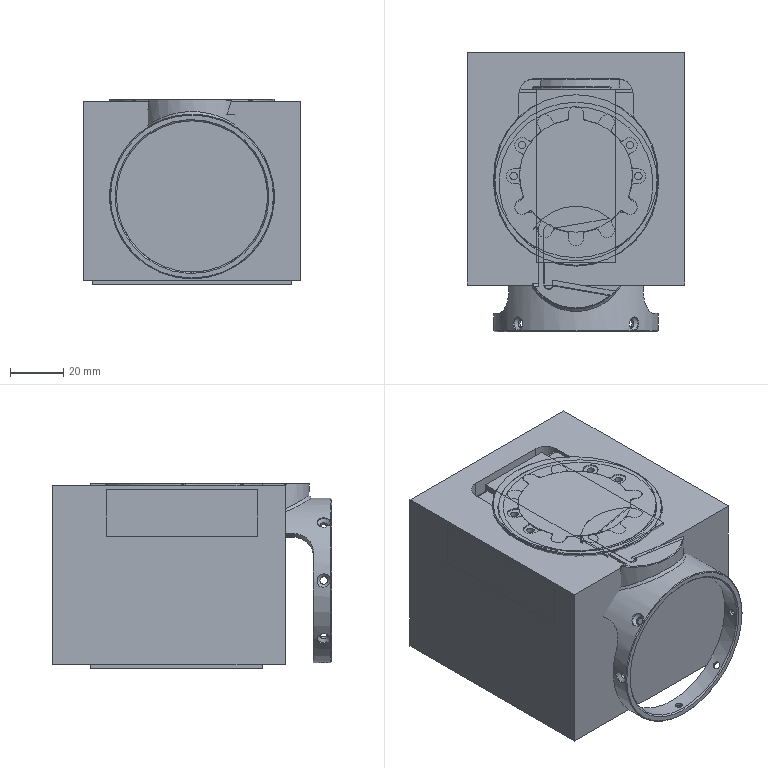NC program | NX | posted with a generic post | part box 82 x 105.2 x 70 mm
Lines 1 to 900 of 123648:
N10 G17 G21 G94 G90
(单向轮廓精光_2 , TOOL : 飞刀D50)
N12 T20 M6
N14 G53
N16 G17 G0 G90 X-63.629 Y-5.85 S5500 M3
N18 G43 Z40.05 H20
N20 Z3.05
N22 G94 G1 Z0.05 F800.
N24 G41 X-51.5 D20
N26 G3 X-48.5 Y-2.85 R3.
N28 G2 X0. Y45.65 R48.5
N30 X-48.5 Y-2.85 R-48.5
N32 X-48.497 Y-2.35 R48.5
N34 G3 X-51.466 Y0.681 R3.
N36 G1 X-63.395 Y0.804
N38 G40
N40 X-63.595 Y0.806
N42 Z3.05
N44 G0 Z40.05
N46 M5
(外形动态铣 , TOOL : 粗刀D16)
N48 T18 M6
N50 G53
N52 G17 G0 G90 X-43.842 Y-2.841 S8500 M3
N54 G43 Z43.08 H18
N56 G94 G1 Z-36.92 F4500.
N58 Z-37.92
N60 X-41.377 Y-3.256
N62 G3 X-40.531 Y-2.841 R0.808
N64 X-40.076 Y-1.778 R5.051
N66 X-39.508 Y1.018 R16.6
N68 X-39.175 Y5.411 R51.899
N70 X-39.062 Y10.142 R137.49
N72 X-39. Y23.191 R842.38
N74 G1 X-38.997 Y33.828
N76 G2 X-38.706 Y36.242 R9.777
N78 X-36.994 Y39.327 R7.332
N80 X-34.009 Y41.563 R10.476
N82 X-30.312 Y42.892 R16.459
N84 X-25.684 Y43.606 R32.132
N86 X-19.505 Y43.912 R90.843
N88 X-7.131 Y43.999 R599.853
N90 G1 X28.819 Y43.997
N92 G2 X31.234 Y43.711 R10.059
N94 X34.021 Y42.218 R7.173
N96 X36.263 Y39.468 R10.133
N98 X37.731 Y35.826 R15.468
N100 X38.524 Y31.402 R28.5
N102 X38.891 Y25.227 R77.968
N104 X38.996 Y14.54 R445.482
N106 G1 X38.999 Y0.986
N108 G2 X39.12 Y-5.181 R38.622
N110 G3 X39.011 Y-14.829 R391.76
N112 G2 X39.006 Y-18.198 R174.731
N114 G1 X38.996 Y-33.89
N116 G2 X38.692 Y-36.301 R9.598
N118 X37.289 Y-38.928 R7.164
N120 X34.571 Y-41.203 R10.136
N122 X31.121 Y-42.648 R15.035
N124 X26.703 Y-43.49 R27.258
N126 X21.28 Y-43.858 R66.36
N128 X13.594 Y-43.983 R258.777
N130 X5.719 Y-43.999 R1000.
N132 G1 X-28.731 Y-43.998
N134 G2 X-31.149 Y-43.735 R10.493
N136 X-34.096 Y-42.155 R7.16
N138 X-36.217 Y-39.55 R10.128
N140 X-37.709 Y-35.911 R15.308
N142 X-38.515 Y-31.489 R28.138
N144 X-38.878 Y-25.689 R73.44
N146 X-38.985 Y-18.378 R277.454
N148 X-38.992 Y-7.74 R1000.
N150 G1 X-38.962 Y-7.053
N152 G2 X-38.286 Y5.503 R39.004
N154 G3 X-37.805 Y9.676 R36.79
N156 X-37.638 Y13.604 R77.844
N158 X-37.516 Y21.71 R298.384
N160 X-37.498 Y30.316 R1000.
N162 G2 X-37.024 Y33.454 R9.775
N164 X-34.408 Y37.509 R9.889
N166 X-30.998 Y39.83 R13.575
N168 X-26.565 Y41.325 R20.601
N170 X-21.374 Y42.081 R39.28
N172 X-17.257 Y42.331 R68.099
N174 X-7.509 Y42.483 R307.632
N176 G1 X1.866 Y42.498
N178 X25.377 Y42.496
N180 G2 X31.311 Y40.453 R9.474
N182 X34.146 Y37.208 R12.
N184 X35.917 Y33.085 R17.353
N186 X36.916 Y27.937 R31.063
N188 X37.344 Y21.766 R77.264
N190 X37.487 Y12.393 R315.161
N192 G1 X37.496 Y8.643
N194 X37.525 Y8.434
N196 G2 X39. Y0.977 R38.909
N198 X39.12 Y-5.181 R38.636
N200 X38.217 Y-11.508 R38.847
N202 G3 X37.78 Y-15.358 R34.515
N204 X37.581 Y-20.728 R123.29
N206 X37.499 Y-30.573 R690.567
N208 G2 X35.467 Y-36.302 R9.461
N210 X32.198 Y-39.158 R12.015
N212 X27.892 Y-40.977 R17.621
N214 X22.924 Y-41.918 R31.934
N216 X16.378 Y-42.357 R79.079
N218 X6.066 Y-42.489 R346.547
N220 G1 X-4.809 Y-42.499
N222 X-25.377 Y-42.496
N224 G2 X-31.295 Y-40.469 R9.472
N226 X-34.156 Y-37.198 R12.011
N228 X-35.976 Y-32.893 R17.625
N230 X-36.918 Y-27.925 R31.867
N232 X-37.352 Y-21.566 R77.779
N234 X-37.473 Y-14.443 R267.157
N236 G1 X-37.5 Y-14.223
N238 G2 X-38.97 Y-6.979 R39.227
N240 G3 X-37.501 Y-14.222 R39.229
N242 G1 X-37.157 Y-15.308
N244 X-36.969 Y-15.838
N246 G2 X-36.371 Y-18.766 R19.993
N248 X-35.945 Y-22.645 R79.694
N250 G3 X-35.379 Y-27.487 R89.613
N252 X-34.437 Y-31.69 R27.733
N254 X-32.981 Y-34.931 R14.06
N256 X-30.112 Y-37.849 R9.443
N258 X-26.555 Y-39.507 R14.108
N260 X-22.342 Y-40.406 R24.559
N262 X-16.924 Y-40.832 R60.218
N264 X-9.06 Y-40.975 R240.729
N266 X6.368 Y-41.514 R38.987
N268 G2 X10.854 Y-41.127 R58.127
N270 X16.044 Y-40.884 R709.084
N272 G3 X21.837 Y-40.417 R78.068
N274 X26.247 Y-39.548 R29.517
N276 X29.7 Y-38.107 R15.061
N278 X32.714 Y-35.307 R9.485
N280 X34.443 Y-31.776 R13.67
N282 X35.427 Y-27.39 R24.896
N284 X35.915 Y-21.976 R69.432
N286 G1 X36.127 Y-18.166
N288 X36.171 Y-17.919
N290 G3 X38.217 Y-11.508 R38.238
N292 G2 X36.171 Y-17.919 R38.238
N294 G1 X35.901 Y-18.565
N296 X35.855 Y-18.669
N298 X35.698 Y-19.01
N300 G3 X35.005 Y-21.434 R16.049
N302 X34.298 Y-25.29 R89.694
N304 G2 X33.46 Y-28.943 R33.503
N306 X32.297 Y-31.701 R12.849
N308 X29.159 Y-35.187 R11.86
N310 X25.021 Y-37.392 R16.188
N312 X20.31 Y-38.62 R26.777
N314 X14.914 Y-39.274 R63.287
N316 G3 X14.276 Y-39.345 R5.23
N318 G2 X6.318 Y-41.523 R39.048
N320 G3 X14.276 Y-39.345 R39.048
N322 G1 X15.227 Y-38.959
N324 X15.77 Y-38.723
N326 X15.941 Y-38.646
N328 G2 X18.187 Y-37.891 R25.953
N330 G3 X21.423 Y-36.912 R124.592
N332 X24.724 Y-35.581 R24.909
N334 X29.589 Y-31.221 R12.715
N336 X31.176 Y-28.248 R16.816
N338 X32.253 Y-25.243 R32.204
N340 G2 X32.407 Y-24.88 R1.724
N342 G3 X35.704 Y-18.996 R38.411
N344 G2 X32.407 Y-24.88 R38.411
N346 X30.853 Y-27.01 R39.013
N348 X29.161 Y-29.231 R51.949
N350 X25.724 Y-32.414 R17.082
N352 X15.799 Y-38.71 R39.068
N354 G3 X25.724 Y-32.414 R39.068
N356 X30.896 Y-26.956 R38.689
N358 G2 X31.658 Y-26.664 R0.8
N360 G1 X32.192 Y-26.755
N362 X34.755 Y-27.193 Z-37.42
N364 X35.973 Y-27.397 F15000.
N366 G3 X36.746 Y-26.956 R0.801
N368 G1 X37.421 Y-25.608
N370 X38.067 Y-24.245
N372 X38.431 Y-23.392
N374 X38.774 Y-22.53
N376 X40.517 Y-17.908
N378 G3 X42.826 Y-9.272 R51.615
N380 X43.242 Y-3.556 R31.236
N382 X42.919 Y2.276 R64.812
N384 G1 X42.58 Y5.586
N386 G3 X42.109 Y6.165 R0.802
N388 G1 X41.405 Y6.465
N390 X39.014 Y7.484 Z-37.92 F4500.
N392 X37.979 Y7.925
N394 G2 X37.525 Y8.434 R0.8
N396 G1 X37.483 Y8.577
N398 X37.315 Y9.12
N400 X37.017 Y10.009
N402 G2 X36.443 Y12.984 R18.568
N404 X36.135 Y16.77 R51.586
N406 G1 X35.811 Y22.518
N408 G3 X35.32 Y27.555 R62.222
N410 X34.392 Y31.761 R26.311
N412 X33.117 Y34.678 R14.269
N414 X29.567 Y38.207 R9.713
N416 X25.757 Y39.756 R15.175
N418 X21.33 Y40.534 R28.963
N420 X17.215 Y40.824 R63.587
N422 G2 X16.807 Y40.9 R1.936
N424 G3 X15.227 Y41.585 R17.313
N426 X12.513 Y42.04 R8.19
N428 G1 X-15.715
N430 G3 X-18.429 Y41.598 R8.452
N432 G2 X-21.262 Y40.914 R38.186
N434 G3 X-24.56 Y40.188 R89.188
N436 X-28.292 Y38.95 R22.946
N438 X-31.007 Y37.299 R11.587
N440 X-33.349 Y34.396 R10.433
N442 X-34.777 Y30.737 R15.811
N444 X-35.55 Y26.309 R29.629
N446 X-35.915 Y20.697 R83.832
N448 G1 X-36.136 Y13.875
N450 X-36.211 Y12.242
N452 X-36.258 Y12.019
N454 G3 X-38.287 Y5.497 R38.808
N456 G2 X-36.258 Y12.019 R38.808
N458 G1 X-36.111 Y12.377
N460 X-35.877 Y12.92
N462 X-35.8 Y13.091
N464 G3 X-35.159 Y15.558 R14.732
N466 X-34.699 Y19.214 R40.224
N468 G2 X-34.24 Y24.02 R653.097
N470 X-33.593 Y28.091 R35.456
N472 X-32.583 Y31.108 R14.57
N474 X-29.609 Y34.925 R11.558
N476 X-25.956 Y37.249 R16.559
N478 X-22.821 Y38.517 R31.938
N480 G3 X-22.469 Y38.756 R1.94
N482 G2 X-21.144 Y40.083 R11.617
N484 X-18.972 Y41.395 R8.952
N486 G1 X-18.429 Y41.598
N488 G3 X-20.601 Y40.498 R8.734
N490 X-21.759 Y39.519 R9.573
N492 X-22.469 Y38.756 R10.8
N494 G1 X-22.743 Y38.433
N496 G2 X-23.943 Y37.387 R11.134
N498 G3 X-26.289 Y35.565 R140.424
N500 X-30.5 Y30.038 R15.149
N502 X-31.93 Y25.778 R23.539
N504 X-32.735 Y21.542 R50.637
N506 G2 X-33.281 Y18.013 R289.28
N508 X-33.41 Y17.632 R1.818
N510 G3 X-35.864 Y12.949 R38.871
N512 G2 X-33.41 Y17.632 R38.871
N514 G1 X-33.305 Y17.805
N516 X-33.086 Y18.154
N518 X-32.962 Y18.348
N520 G3 X-32.16 Y20.139 R11.443
N522 X-31.324 Y22.746 R49.15
N524 G2 X-30.295 Y25.967 R57.976
N526 X-28.92 Y29.045 R21.11
N528 X-26.122 Y32.83 R20.308
N530 X-24.683 Y34.33 R53.77
N532 G3 X-24.451 Y34.73 R1.889
N534 G2 X-22.743 Y38.433 R8.946
N536 G3 X-24.451 Y34.73 R8.946
N538 G2 X-24.719 Y34.205 R0.922
N540 G3 X-26.029 Y32.794 R12.537
N542 X-27.318 Y30.291 R8.392
N544 G1 X-28.527 Y26.572
N546 G2 X-29.755 Y22.739 R243.657
N548 G1 X-29.87 Y22.52
N550 G3 X-32.962 Y18.348 R39.117
N552 G2 X-29.87 Y22.52 R39.117
N554 G1 X-29.829 Y22.568
N556 X-29.724 Y22.691
N558 X-29.353 Y23.114
N560 G3 X-28.253 Y24.822 R11.45
N562 X-27.789 Y25.729 R21.099
N564 X-27.69 Y26.129 R1.917
N566 G1 Y27.576
N568 G2 X-27.318 Y30.291 R8.585
N570 G3 X-27.69 Y27.576 R8.585
N572 G1 Y26.129
N574 G2 X-27.697 Y25.133 R18.125
N576 X-27.946 Y24.623 R0.894
N578 G3 X-29.372 Y23.093 R33.212
N580 G2 X-30.103 Y22.83 R0.8
N582 G1 X-30.805 Y22.944
N584 X-33.371 Y23.361 Z-37.42
N586 X-34.456 Y23.533 F15000.
N588 G3 X-35.222 Y23.093 R0.801
N590 G1 X-39.06 Y15.409
N592 G3 X-41.21 Y9.78 R37.478
N594 X-42.291 Y5.945 R82.679
N596 X-43.121 Y1.899 R52.322
N598 G1 X-43.617 Y-1.154
N600 G3 X-43.24 Y-8.178 R18.119
N602 G1 X-42.012 Y-12.989
N604 G3 X-41.595 Y-13.443 R0.805
N606 G1 X-41.03 Y-13.703
N608 X-38.668 Y-14.79 Z-37.92 F4500.
N610 X-37.389 Y-15.378
N612 G2 X-36.969 Y-15.838 R0.8
N614 G3 X-35.832 Y-18.709 R36.832
N616 G2 X-35.098 Y-21.153 R17.073
N618 X-34.278 Y-25.345 R90.908
N620 G3 X-33.374 Y-29.179 R35.936
N622 X-29.298 Y-35.106 R11.695
N624 X-25.371 Y-37.302 R15.535
N626 X-21.221 Y-38.474 R23.966
N628 X-16.202 Y-39.119 R44.455
N630 G1 X-14.706 Y-39.221
N632 X-14.482 Y-39.263
N634 G3 X-9.018 Y-40.984 R38.563
N636 G2 X-14.482 Y-39.263 R38.563
N638 G1 X-14.663 Y-39.193
N640 X-15.172 Y-38.979
N642 X-15.942 Y-38.65
N644 G3 X-18.161 Y-37.911 R23.584
N646 G2 X-21.57 Y-36.891 R103.263
N648 X-24.528 Y-35.71 R25.389
N650 X-29.641 Y-31.147 R12.792
N652 X-31.285 Y-27.987 R17.602
N654 X-32.291 Y-25.155 R35.025
N656 G1 X-32.382 Y-24.916
N658 G2 X-35.883 Y-18.593 R38.238
N660 G3 X-32.382 Y-24.916 R38.238
N662 X-30.74 Y-27.151 R36.227
N664 X-29.055 Y-29.363 R46.055
N666 X-25.607 Y-32.514 R17.129
N668 X-15.942 Y-38.65 R39.376
N670 G2 X-25.607 Y-32.514 R39.376
N672 X-30.778 Y-27.103 R38.488
N674 G3 X-31.543 Y-26.808 R0.8
N676 G1 X-32.093 Y-26.902
N678 X-34.656 Y-27.341 Z-37.42
N680 X-35.855 Y-27.543 F15000.
N682 G2 X-36.628 Y-27.103 R0.801
N684 G1 X-37.303 Y-25.754
N686 X-37.949 Y-24.392
N688 X-38.313 Y-23.538
N690 X-38.656 Y-22.676
N692 X-40.4 Y-18.055
N694 G2 X-42.616 Y-9.844 R48.652
N696 X-43.128 Y-3.782 R36.214
N698 G1 X-43.124 Y1.713
N700 G2 X-41.61 Y9.192 R21.229
N702 X-34.22 Y25.727 R203.286
N704 G1 X-33.233 Y27.656
N706 X-29.237 Y35.347
N708 G2 X-26.064 Y40.364 R41.323
N710 G1 X-25.438 Y41.217
N712 X-24.796 Y42.059
N714 G2 X-22.217 Y44.193 R9.185
N716 X-16.17 Y45.953 R13.105
N718 X-13.465 Y46.033 R44.97
N720 G1 X13.959 Y45.963
N722 G2 X14.614 Y45.485 R0.801
N724 G1 X14.794 Y45.069
N726 X15.828 Y42.684 Z-37.92 F4500.
N728 X16.428 Y41.299
N730 G3 X16.807 Y40.9 R0.8
N732 G1 X16.855 Y40.878
N734 X17.358 Y40.605
N736 G3 X19.445 Y39.857 R13.469
N738 X22.422 Y39.07 R294.444
N740 G2 X25.267 Y38.127 R22.709
N742 X30.207 Y34.213 R11.821
N744 X32.395 Y30.086 R16.44
N746 X33.59 Y25.559 R26.867
N748 X34.251 Y20.541 R61.123
N750 G3 X34.678 Y15.858 R615.575
N752 X34.755 Y15.32 R3.149
N754 G1 X34.824 Y15.126
N756 G2 X37.06 Y9.88 R38.322
N758 G3 X34.824 Y15.126 R38.322
N760 G1 X34.769 Y15.232
N762 X34.557 Y15.634
N764 X34.377 Y15.963
N766 G2 X33.619 Y18.112 R12.322
N768 X32.815 Y21.813 R52.002
N770 G3 X31.869 Y26.019 R58.267
N772 X30.513 Y29.71 R21.204
N774 X26.277 Y34.661 R12.921
N776 X22.685 Y36.678 R21.709
N778 X20.516 Y37.622 R78.616
N780 G2 X20.076 Y37.992 R1.371
N782 G3 X17.358 Y40.605 R8.32
N784 G2 X20.076 Y37.992 R8.32
N786 G1 X20.112 Y37.939
N788 X20.143 Y37.89
N790 X20.236 Y37.728
N792 G3 X21.33 Y36.656 R7.845
N794 X23.179 Y35.19 R110.759
N796 G2 X24.633 Y34.091 R8.721
N798 X25.692 Y33.005 R23.132
N800 X28.891 Y28.12 R18.838
N802 X30.233 Y24.607 R28.391
N804 X31.306 Y20.873 R87.62
N806 G3 X31.469 Y20.501 R1.868
N808 G2 X34.406 Y15.91 R38.12
N810 G3 X31.469 Y20.501 R38.12
N812 G1 X30.969 Y21.163
N814 X30.854 Y21.311
N816 G2 X29.707 Y23.247 R16.241
N818 G3 X28.064 Y26.421 R177.252
N820 G1 X27.79 Y26.912
N822 G2 X27.685 Y27.315 R1.937
N824 G3 X27.412 Y29.748 R8.968
N826 X25.692 Y33.005 R8.352
N828 G2 X27.671 Y28.119 R8.275
N830 G1 X27.685 Y27.315
N832 X27.686 Y26.94
N834 G3 X27.972 Y25.174 R8.361
N836 X28.197 Y24.448 R5.127
N838 G1 X28.325 Y24.232
N840 G2 X30.854 Y21.31 R37.881
N842 G3 X28.325 Y24.232 R37.881
N844 G2 X27.867 Y24.713 R25.124
N846 X27.687 Y25.251 R0.894
N848 G1 X27.685 Y27.126
N850 G3 X27.622 Y28.662 R11.469
N852 X25.18 Y33.548 R8.269
N854 X23.999 Y34.633 R12.001
N856 X23.179 Y35.19 R9.986
N858 X21.741 Y35.866 R8.334
N860 G1 X21.438 Y36.003
N862 G2 X20.871 Y36.472 R1.133
N864 G1 X20.812 Y36.553
N866 G3 X20.174 Y37.836 R7.903
N868 G2 X20.812 Y36.553 R7.903
N870 G3 X21.394 Y35.976 R0.902
N872 G1 X21.741 Y35.866
N874 G3 X22.707 Y36.273 R0.808
N876 G1 X23.833 Y38.512
N878 Z-36.92
N880 G0 Z43.08
N882 X-43.842 Y-2.841
N884 G1 Z-65.
N886 Z-66.
N888 X-41.377 Y-3.256
N890 G3 X-40.531 Y-2.841 R0.808
N892 X-40.076 Y-1.778 R5.051
N894 X-39.508 Y1.018 R16.6
N896 X-39.175 Y5.411 R51.899
N898 X-39.062 Y10.142 R137.49
N900 X-39. Y23.191 R842.38
N902 G1 X-38.997 Y33.828
N904 G2 X-38.706 Y36.242 R9.777
N906 X-36.994 Y39.327 R7.332
N908 X-34.009 Y41.563 R10.476
N910 X-30.312 Y42.892 R16.459
N912 X-25.684 Y43.606 R32.132
N914 X-19.505 Y43.912 R90.843
N916 X-7.131 Y43.999 R599.853
N918 G1 X28.819 Y43.997
N920 G2 X31.234 Y43.711 R10.059
N922 X34.021 Y42.218 R7.173
N924 X36.263 Y39.468 R10.133
N926 X37.731 Y35.826 R15.468
N928 X38.524 Y31.402 R28.5
N930 X38.891 Y25.227 R77.968
N932 X38.996 Y14.54 R445.482
N934 G1 X38.999 Y0.986
N936 G2 X39.12 Y-5.181 R38.622
N938 G3 X39.011 Y-14.829 R391.76
N940 G2 X39.006 Y-18.198 R174.731
N942 G1 X38.996 Y-33.89
N944 G2 X38.692 Y-36.301 R9.598
N946 X37.289 Y-38.928 R7.164
N948 X34.571 Y-41.203 R10.136
N950 X31.121 Y-42.648 R15.035
N952 X26.703 Y-43.49 R27.258
N954 X21.28 Y-43.858 R66.36
N956 X13.594 Y-43.983 R258.777
N958 X5.719 Y-43.999 R1000.
N960 G1 X-28.731 Y-43.998
N962 G2 X-31.149 Y-43.735 R10.493
N964 X-34.096 Y-42.155 R7.16
N966 X-36.217 Y-39.55 R10.128
N968 X-37.709 Y-35.911 R15.308
N970 X-38.515 Y-31.489 R28.138
N972 X-38.878 Y-25.689 R73.44
N974 X-38.985 Y-18.378 R277.454
N976 X-38.992 Y-7.74 R1000.
N978 G1 X-38.962 Y-7.053
N980 G2 X-38.286 Y5.503 R39.004
N982 G3 X-37.805 Y9.676 R36.79
N984 X-37.638 Y13.604 R77.844
N986 X-37.516 Y21.71 R298.384
N988 X-37.498 Y30.316 R1000.
N990 G2 X-37.024 Y33.454 R9.775
N992 X-34.408 Y37.509 R9.889
N994 X-30.998 Y39.83 R13.575
N996 X-26.565 Y41.325 R20.601
N998 X-21.374 Y42.081 R39.28
N1000 X-17.257 Y42.331 R68.099
N1002 X-7.509 Y42.483 R307.632
N1004 G1 X1.866 Y42.498
N1006 X25.377 Y42.496
N1008 G2 X31.311 Y40.453 R9.474
N1010 X34.146 Y37.208 R12.
N1012 X35.917 Y33.085 R17.353
N1014 X36.916 Y27.937 R31.063
N1016 X37.344 Y21.766 R77.264
N1018 X37.487 Y12.393 R315.161
N1020 G1 X37.496 Y8.643
N1022 X37.525 Y8.434
N1024 G2 X39. Y0.977 R38.909
N1026 X39.12 Y-5.181 R38.636
N1028 X38.217 Y-11.508 R38.847
N1030 G3 X37.78 Y-15.358 R34.515
N1032 X37.581 Y-20.728 R123.29
N1034 X37.499 Y-30.573 R690.567
N1036 G2 X35.467 Y-36.302 R9.461
N1038 X32.198 Y-39.158 R12.015
N1040 X27.892 Y-40.977 R17.621
N1042 X22.924 Y-41.918 R31.934
N1044 X16.378 Y-42.357 R79.079
N1046 X6.066 Y-42.489 R346.547
N1048 G1 X-4.809 Y-42.499
N1050 X-25.377 Y-42.496
N1052 G2 X-31.295 Y-40.469 R9.472
N1054 X-34.156 Y-37.198 R12.011
N1056 X-35.976 Y-32.893 R17.625
N1058 X-36.918 Y-27.925 R31.867
N1060 X-37.352 Y-21.566 R77.779
N1062 X-37.473 Y-14.443 R267.157
N1064 G1 X-37.5 Y-14.223
N1066 G2 X-38.97 Y-6.979 R39.227
N1068 G3 X-37.501 Y-14.222 R39.229
N1070 G1 X-37.157 Y-15.308
N1072 X-36.969 Y-15.838
N1074 G2 X-36.371 Y-18.766 R19.993
N1076 X-35.945 Y-22.645 R79.694
N1078 G3 X-35.379 Y-27.487 R89.613
N1080 X-34.437 Y-31.69 R27.733
N1082 X-32.981 Y-34.931 R14.06
N1084 X-30.112 Y-37.849 R9.443
N1086 X-26.555 Y-39.507 R14.108
N1088 X-22.342 Y-40.406 R24.559
N1090 X-16.924 Y-40.832 R60.218
N1092 X-9.06 Y-40.975 R240.729
N1094 X6.368 Y-41.514 R38.987
N1096 G2 X10.854 Y-41.127 R58.127
N1098 X16.044 Y-40.884 R709.084
N1100 G3 X21.837 Y-40.417 R78.068
N1102 X26.247 Y-39.548 R29.517
N1104 X29.7 Y-38.107 R15.061
N1106 X32.714 Y-35.307 R9.485
N1108 X34.443 Y-31.776 R13.67
N1110 X35.427 Y-27.39 R24.896
N1112 X35.915 Y-21.976 R69.432
N1114 G1 X36.127 Y-18.166
N1116 X36.171 Y-17.919
N1118 G3 X38.217 Y-11.508 R38.238
N1120 G2 X36.171 Y-17.919 R38.238
N1122 G1 X35.901 Y-18.565
N1124 X35.855 Y-18.669
N1126 X35.698 Y-19.01
N1128 G3 X35.005 Y-21.434 R16.049
N1130 X34.298 Y-25.29 R89.694
N1132 G2 X33.46 Y-28.943 R33.503
N1134 X32.297 Y-31.701 R12.849
N1136 X29.159 Y-35.187 R11.86
N1138 X25.021 Y-37.392 R16.188
N1140 X20.31 Y-38.62 R26.777
N1142 X14.914 Y-39.274 R63.287
N1144 G3 X14.276 Y-39.345 R5.23
N1146 G2 X6.318 Y-41.523 R39.048
N1148 G3 X14.276 Y-39.345 R39.048
N1150 G1 X15.227 Y-38.959
N1152 X15.77 Y-38.723
N1154 X15.941 Y-38.646
N1156 G2 X18.187 Y-37.891 R25.953
N1158 G3 X21.423 Y-36.912 R124.592
N1160 X24.724 Y-35.581 R24.909
N1162 X29.589 Y-31.221 R12.715
N1164 X31.176 Y-28.248 R16.816
N1166 X32.253 Y-25.243 R32.204
N1168 G2 X32.407 Y-24.88 R1.724
N1170 G3 X35.704 Y-18.996 R38.411
N1172 G2 X32.407 Y-24.88 R38.411
N1174 X30.853 Y-27.01 R39.013
N1176 X29.161 Y-29.231 R51.949
N1178 X25.724 Y-32.414 R17.082
N1180 X15.799 Y-38.71 R39.068
N1182 G3 X25.724 Y-32.414 R39.068
N1184 X30.896 Y-26.956 R38.689
N1186 G2 X31.658 Y-26.664 R0.8
N1188 G1 X32.192 Y-26.755
N1190 X34.755 Y-27.193 Z-65.5
N1192 X35.973 Y-27.397 F15000.
N1194 G3 X36.746 Y-26.956 R0.801
N1196 G1 X37.421 Y-25.608
N1198 X38.067 Y-24.245
N1200 X38.431 Y-23.392
N1202 X38.774 Y-22.53
N1204 X40.517 Y-17.908
N1206 G3 X42.826 Y-9.272 R51.615
N1208 X43.242 Y-3.556 R31.236
N1210 X42.919 Y2.276 R64.812
N1212 G1 X42.58 Y5.586
N1214 G3 X42.109 Y6.165 R0.802
N1216 G1 X41.405 Y6.465
N1218 X39.014 Y7.484 Z-66. F4500.
N1220 X37.979 Y7.925
N1222 G2 X37.525 Y8.434 R0.8
N1224 G1 X37.483 Y8.577
N1226 X37.315 Y9.12
N1228 X37.017 Y10.009
N1230 G2 X36.443 Y12.984 R18.568
N1232 X36.135 Y16.77 R51.586
N1234 G1 X35.811 Y22.518
N1236 G3 X35.32 Y27.555 R62.222
N1238 X34.392 Y31.761 R26.311
N1240 X33.117 Y34.678 R14.269
N1242 X29.567 Y38.207 R9.713
N1244 X25.757 Y39.756 R15.175
N1246 X21.33 Y40.534 R28.963
N1248 X17.215 Y40.824 R63.587
N1250 G2 X16.807 Y40.9 R1.936
N1252 G3 X15.227 Y41.585 R17.313
N1254 X12.513 Y42.04 R8.19
N1256 G1 X-15.715
N1258 G3 X-18.429 Y41.598 R8.452
N1260 G2 X-21.262 Y40.914 R38.186
N1262 G3 X-24.56 Y40.188 R89.188
N1264 X-28.292 Y38.95 R22.946
N1266 X-31.007 Y37.299 R11.587
N1268 X-33.349 Y34.396 R10.433
N1270 X-34.777 Y30.737 R15.811
N1272 X-35.55 Y26.309 R29.629
N1274 X-35.915 Y20.697 R83.832
N1276 G1 X-36.136 Y13.875
N1278 X-36.211 Y12.242
N1280 X-36.258 Y12.019
N1282 G3 X-38.287 Y5.497 R38.808
N1284 G2 X-36.258 Y12.019 R38.808
N1286 G1 X-36.111 Y12.377
N1288 X-35.877 Y12.92
N1290 X-35.8 Y13.091
N1292 G3 X-35.159 Y15.558 R14.731
N1294 X-34.699 Y19.214 R40.223
N1296 G2 X-34.24 Y24.02 R653.167
N1298 X-33.593 Y28.091 R35.456
N1300 X-32.583 Y31.108 R14.57
N1302 X-29.609 Y34.925 R11.558
N1304 X-25.956 Y37.249 R16.559
N1306 X-22.821 Y38.517 R31.938
N1308 G3 X-22.469 Y38.756 R1.94
N1310 G2 X-21.144 Y40.083 R11.616
N1312 X-18.972 Y41.395 R8.952
N1314 G1 X-18.429 Y41.598
N1316 G3 X-20.601 Y40.498 R8.734
N1318 X-21.759 Y39.519 R9.573
N1320 X-22.469 Y38.756 R10.796
N1322 G1 X-22.743 Y38.433
N1324 G2 X-23.943 Y37.387 R11.134
N1326 G3 X-26.289 Y35.565 R140.424
N1328 X-30.5 Y30.038 R15.149
N1330 X-31.93 Y25.778 R23.539
N1332 X-32.735 Y21.542 R50.637
N1334 G2 X-33.281 Y18.013 R289.264
N1336 X-33.41 Y17.632 R1.818
N1338 G3 X-35.864 Y12.949 R38.895
N1340 G2 X-33.41 Y17.632 R38.895
N1342 G1 X-33.305 Y17.805
N1344 X-33.086 Y18.154
N1346 X-32.962 Y18.348
N1348 G3 X-32.16 Y20.139 R11.443
N1350 X-31.324 Y22.746 R49.15
N1352 G2 X-30.295 Y25.967 R57.976
N1354 X-28.92 Y29.045 R21.11
N1356 X-26.122 Y32.83 R20.308
N1358 X-24.683 Y34.33 R53.77
N1360 G3 X-24.451 Y34.73 R1.889
N1362 G2 X-22.743 Y38.433 R8.946
N1364 G3 X-24.451 Y34.73 R8.946
N1366 G2 X-24.719 Y34.205 R0.922
N1368 G3 X-26.029 Y32.794 R12.537
N1370 X-27.318 Y30.291 R8.392
N1372 G1 X-28.527 Y26.572
N1374 G2 X-29.755 Y22.739 R243.657
N1376 G1 X-29.87 Y22.52
N1378 G3 X-32.962 Y18.348 R39.117
N1380 G2 X-29.87 Y22.52 R39.117
N1382 G1 X-29.829 Y22.568
N1384 X-29.724 Y22.691
N1386 X-29.353 Y23.114
N1388 G3 X-28.253 Y24.822 R11.45
N1390 X-27.789 Y25.729 R21.099
N1392 X-27.69 Y26.129 R1.917
N1394 G1 Y27.576
N1396 G2 X-27.318 Y30.291 R8.585
N1398 G3 X-27.69 Y27.576 R8.585
N1400 G1 Y26.129
N1402 G2 X-27.697 Y25.133 R18.125
N1404 X-27.946 Y24.623 R0.894
N1406 G3 X-29.372 Y23.093 R33.212
N1408 G2 X-30.103 Y22.83 R0.8
N1410 G1 X-30.805 Y22.944
N1412 X-33.371 Y23.361 Z-65.5
N1414 X-34.456 Y23.533 F15000.
N1416 G3 X-35.222 Y23.093 R0.801
N1418 G1 X-39.06 Y15.409
N1420 G3 X-41.21 Y9.78 R37.478
N1422 X-42.291 Y5.945 R82.679
N1424 X-43.121 Y1.899 R52.322
N1426 G1 X-43.617 Y-1.154
N1428 G3 X-43.24 Y-8.178 R18.119
N1430 G1 X-42.012 Y-12.989
N1432 G3 X-41.595 Y-13.443 R0.805
N1434 G1 X-41.03 Y-13.703
N1436 X-38.668 Y-14.79 Z-66. F4500.
N1438 X-37.389 Y-15.378
N1440 G2 X-36.969 Y-15.838 R0.8
N1442 G3 X-35.832 Y-18.709 R36.832
N1444 G2 X-35.098 Y-21.153 R17.073
N1446 X-34.278 Y-25.345 R90.908
N1448 G3 X-33.374 Y-29.179 R35.936
N1450 X-29.298 Y-35.106 R11.695
N1452 X-25.371 Y-37.302 R15.535
N1454 X-21.221 Y-38.474 R23.966
N1456 X-16.202 Y-39.119 R44.455
N1458 G1 X-14.706 Y-39.221
N1460 X-14.482 Y-39.263
N1462 G3 X-9.018 Y-40.984 R38.563
N1464 G2 X-14.482 Y-39.263 R38.563
N1466 G1 X-14.663 Y-39.193
N1468 X-15.172 Y-38.979
N1470 X-15.942 Y-38.65
N1472 G3 X-18.161 Y-37.911 R23.584
N1474 G2 X-21.57 Y-36.891 R103.263
N1476 X-24.528 Y-35.71 R25.389
N1478 X-29.641 Y-31.147 R12.792
N1480 X-31.285 Y-27.987 R17.602
N1482 X-32.291 Y-25.155 R35.025
N1484 G1 X-32.382 Y-24.916
N1486 G2 X-35.883 Y-18.593 R38.238
N1488 G3 X-32.382 Y-24.916 R38.238
N1490 X-30.74 Y-27.151 R36.227
N1492 X-29.055 Y-29.363 R46.055
N1494 X-25.607 Y-32.514 R17.129
N1496 X-15.942 Y-38.65 R39.376
N1498 G2 X-25.607 Y-32.514 R39.376
N1500 X-30.778 Y-27.103 R38.488
N1502 G3 X-31.543 Y-26.808 R0.8
N1504 G1 X-32.093 Y-26.902
N1506 X-34.656 Y-27.341 Z-65.5
N1508 X-35.855 Y-27.543 F15000.
N1510 G2 X-36.628 Y-27.103 R0.801
N1512 G1 X-37.303 Y-25.754
N1514 X-37.949 Y-24.392
N1516 X-38.313 Y-23.538
N1518 X-38.656 Y-22.676
N1520 X-40.4 Y-18.055
N1522 G2 X-42.616 Y-9.844 R48.652
N1524 X-43.128 Y-3.782 R36.214
N1526 G1 X-43.124 Y1.713
N1528 G2 X-41.61 Y9.192 R21.229
N1530 X-34.22 Y25.727 R203.286
N1532 G1 X-33.233 Y27.656
N1534 X-29.237 Y35.347
N1536 G2 X-26.064 Y40.364 R41.323
N1538 G1 X-25.438 Y41.217
N1540 X-24.796 Y42.059
N1542 G2 X-22.217 Y44.193 R9.185
N1544 X-16.17 Y45.953 R13.105
N1546 X-13.465 Y46.033 R44.97
N1548 G1 X13.959 Y45.963
N1550 G2 X14.614 Y45.485 R0.801
N1552 G1 X14.794 Y45.069
N1554 X15.828 Y42.684 Z-66. F4500.
N1556 X16.428 Y41.299
N1558 G3 X16.807 Y40.9 R0.8
N1560 G1 X16.855 Y40.878
N1562 X17.358 Y40.605
N1564 G3 X19.445 Y39.857 R13.469
N1566 X22.422 Y39.07 R294.444
N1568 G2 X25.267 Y38.127 R22.709
N1570 X30.207 Y34.213 R11.821
N1572 X32.395 Y30.086 R16.44
N1574 X33.59 Y25.559 R26.867
N1576 X34.251 Y20.541 R61.123
N1578 G3 X34.678 Y15.858 R615.575
N1580 X34.755 Y15.32 R3.149
N1582 G1 X34.824 Y15.125
N1584 G2 X37.06 Y9.88 R38.322
N1586 G3 X34.824 Y15.125 R38.322
N1588 G1 X34.769 Y15.232
N1590 X34.557 Y15.634
N1592 X34.377 Y15.963
N1594 G2 X33.619 Y18.112 R12.321
N1596 X32.815 Y21.813 R52.
N1598 G3 X31.869 Y26.019 R58.267
N1600 X30.513 Y29.71 R21.204
N1602 X26.277 Y34.661 R12.921
N1604 X22.685 Y36.678 R21.709
N1606 X20.516 Y37.622 R78.615
N1608 G2 X20.076 Y37.992 R1.371
N1610 G3 X17.358 Y40.605 R8.32
N1612 G2 X20.076 Y37.992 R8.32
N1614 G1 X20.112 Y37.939
N1616 X20.143 Y37.89
N1618 X20.236 Y37.728
N1620 G3 X21.33 Y36.656 R7.845
N1622 X23.179 Y35.19 R110.76
N1624 G2 X24.633 Y34.091 R8.721
N1626 X25.692 Y33.005 R23.132
N1628 X28.891 Y28.12 R18.838
N1630 X30.233 Y24.607 R28.391
N1632 X31.306 Y20.873 R87.621
N1634 G3 X31.469 Y20.501 R1.867
N1636 G2 X34.406 Y15.91 R38.132
N1638 G3 X31.469 Y20.501 R38.132
N1640 G1 X30.969 Y21.163
N1642 X30.854 Y21.311
N1644 G2 X29.707 Y23.247 R16.241
N1646 G3 X28.064 Y26.421 R177.249
N1648 G1 X27.79 Y26.912
N1650 G2 X27.685 Y27.315 R1.938
N1652 G3 X27.412 Y29.748 R8.968
N1654 X25.692 Y33.005 R8.352
N1656 G2 X27.671 Y28.119 R8.275
N1658 G1 X27.685 Y27.315
N1660 X27.686 Y26.94
N1662 G3 X27.972 Y25.174 R8.361
N1664 X28.197 Y24.448 R5.127
N1666 G1 X28.325 Y24.232
N1668 G2 X30.854 Y21.31 R37.881
N1670 G3 X28.325 Y24.232 R37.881
N1672 G2 X27.867 Y24.713 R25.124
N1674 X27.687 Y25.251 R0.894
N1676 G1 X27.685 Y27.126
N1678 G3 X27.622 Y28.662 R11.469
N1680 X25.18 Y33.548 R8.269
N1682 X23.999 Y34.633 R12.001
N1684 X23.179 Y35.19 R9.986
N1686 X21.741 Y35.866 R8.334
N1688 G1 X21.438 Y36.003
N1690 G2 X20.871 Y36.472 R1.133
N1692 G1 X20.812 Y36.553
N1694 G3 X20.174 Y37.836 R7.903
N1696 G2 X20.812 Y36.553 R7.903
N1698 G3 X21.394 Y35.976 R0.902
N1700 G1 X21.741 Y35.866
N1702 G3 X22.707 Y36.273 R0.808
N1704 G1 X23.833 Y38.512
N1706 Z-65.
N1708 G0 Z43.08
(轮廓开粗 , TOOL : 粗刀D16)
N1710 G18 X56.2 Z-69. S5000
N1712 Y-77.5
N1714 Y-36.285
N1716 G1 Y-34.285 F2500.
N1718 G41 X40. D18
N1720 X-40.
N1722 X-56.
N1724 G40
N1726 X-56.2
N1728 Y-36.285
N1730 G0 Y-77.5
N1732 X56.2
N1734 Y-33.07
N1736 G1 Y-31.07
N1738 G41 X40.
N1740 X-40.
N1742 X-56.
N1744 G40
N1746 X-56.2
N1748 Y-33.07
N1750 G0 Y-77.5
N1752 M5
(单向轮廓精光_2_COPY , TOOL : 飞刀D50)
N1754 T20 M6
N1756 G53
N1758 G18 G0 G90 X60.059 Z-28. S5500 M3
N1760 G43 Y73.85 H20
N1762 Y36.85
N1764 G94 G1 Y33.85 F800.
N1766 G41 X19.859 D20
N1768 X-19.859
N1770 X-59.859
N1772 G40
N1774 X-60.059
N1776 Y36.85
N1778 G0 Y73.85
N1780 M5